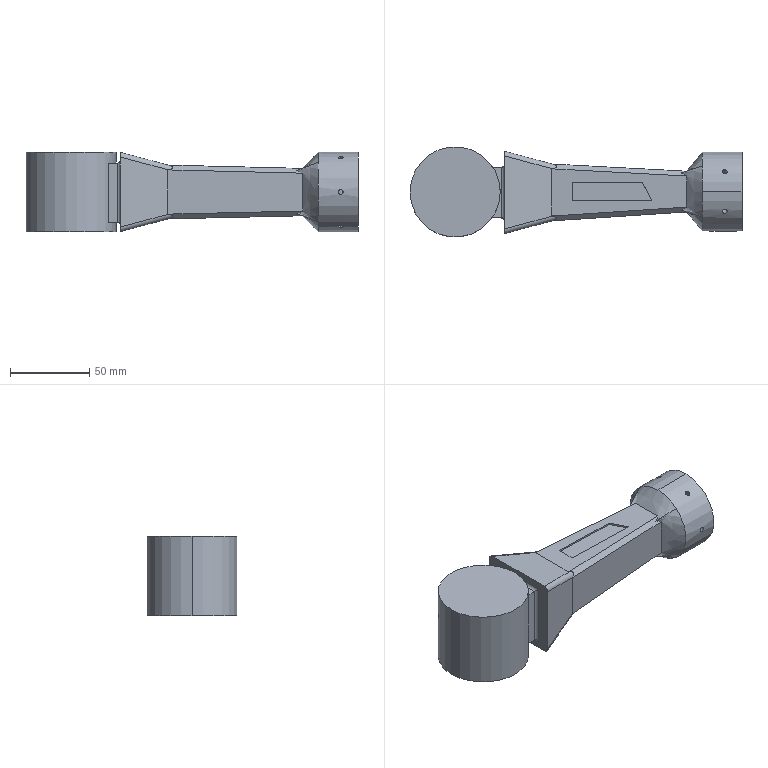Part | SolidWorks | features ICE 6, Blend 2, Fillet 2, Chamfer 1, CirPattern 1, Extrusion 1 | 1 solid | 62 faces | box 209.608 x 56.982 x 50.008 mm | volume 324433 mm3 | plane 26 | cylinder 20 | spline 16 | commonest cylinder face diameters 50 x8 4 x4 6 x4 30 x2 56.982 x2